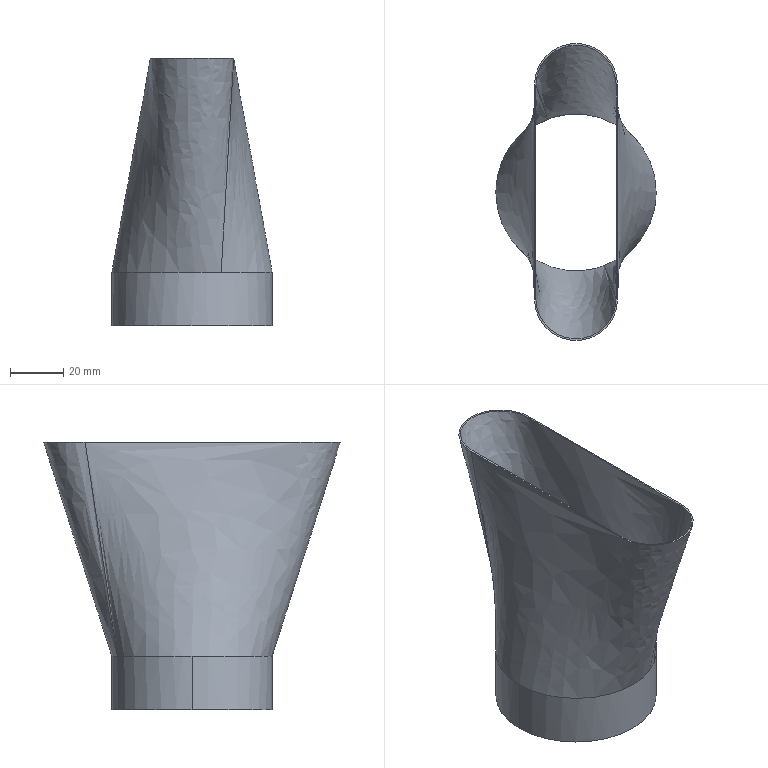Part | SolidWorks | features Blend 1, Extrusion 1, Shell 1 | 1 solid | 12 faces | box 60.001 x 111.2 x 100 mm | volume 12348 mm3 | spline 4 | cylinder 4 | plane 4 | commonest cylinder face diameters 58.8 x2 60 x2